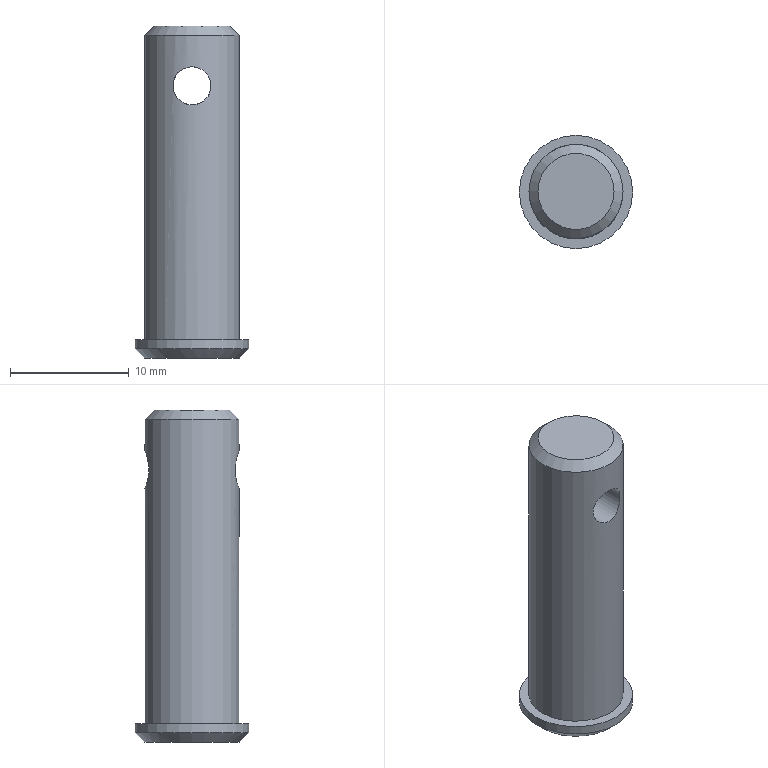Part | NX | features clevis pin, 312 2 | 1 solid | 8 faces | box 9.525 x 9.525 x 27.924 mm | volume 1333 mm3 | plane 3 | cylinder 3 | cone 2 | commonest cylinder face diameters 3.2 x1 7.925 x1 9.525 x1
STEP:
#1=CARTESIAN_POINT('',(4.763,0.,1.524));
#2=VERTEX_POINT('',#1);
#3=CARTESIAN_POINT('',(0.,0.,1.524));
#4=DIRECTION('',(0.,0.,1.));
#5=DIRECTION('',(1.,0.,0.));
#6=AXIS2_PLACEMENT_3D('',#3,#4,#5);
#7=CIRCLE('',#6,4.763);
#8=EDGE_CURVE('',#2,#2,#7,.T.);
#9=ORIENTED_EDGE('',*,*,#8,.T.);
#10=EDGE_LOOP('',(#9));
#11=FACE_BOUND('',#10,.T.);
#12=CARTESIAN_POINT('',(3.962,0.,1.524));
#13=VERTEX_POINT('',#12);
#14=CARTESIAN_POINT('',(0.,0.,1.524));
#15=DIRECTION('',(0.,0.,1.));
#16=DIRECTION('',(1.,0.,0.));
#17=AXIS2_PLACEMENT_3D('',#14,#15,#16);
#18=CIRCLE('',#17,3.962);
#19=EDGE_CURVE('',#13,#13,#18,.T.);
#20=ORIENTED_EDGE('',*,*,#19,.F.);
#21=EDGE_LOOP('',(#20));
#22=FACE_BOUND('',#21,.T.);
#23=CARTESIAN_POINT('',(0.,0.,1.524));
#24=DIRECTION('',(0.,0.,1.));
#25=DIRECTION('',(1.,0.,0.));
#26=AXIS2_PLACEMENT_3D('',#23,#24,#25);
#27=PLANE('',#26);
#28=ADVANCED_FACE('',(#11,#22),#27,.T.);
#29=CARTESIAN_POINT('',(4.763,0.,0.762));
#30=VERTEX_POINT('',#29);
#31=CARTESIAN_POINT('',(0.,0.,0.762));
#32=DIRECTION('',(0.,0.,1.));
#33=DIRECTION('',(1.,0.,0.));
#34=AXIS2_PLACEMENT_3D('',#31,#32,#33);
#35=CIRCLE('',#34,4.763);
#36=EDGE_CURVE('',#30,#30,#35,.T.);
#37=ORIENTED_EDGE('',*,*,#36,.T.);
#38=EDGE_LOOP('',(#37));
#39=FACE_BOUND('',#38,.T.);
#40=ORIENTED_EDGE('',*,*,#8,.F.);
#41=EDGE_LOOP('',(#40));
#42=FACE_BOUND('',#41,.T.);
#43=CARTESIAN_POINT('',(0.,0.,1.524));
#44=DIRECTION('',(0.,0.,-1.));
#45=DIRECTION('',(-1.,0.,0.));
#46=AXIS2_PLACEMENT_3D('',#43,#44,#45);
#47=CYLINDRICAL_SURFACE('',#46,4.763);
#48=ADVANCED_FACE('',(#39,#42),#47,.T.);
#49=CARTESIAN_POINT('',(4.,0.,0.));
#50=VERTEX_POINT('',#49);
#51=CARTESIAN_POINT('',(0.,0.,0.));
#52=DIRECTION('',(0.,0.,1.));
#53=DIRECTION('',(1.,0.,0.));
#54=AXIS2_PLACEMENT_3D('',#51,#52,#53);
#55=CIRCLE('',#54,4.);
#56=EDGE_CURVE('',#50,#50,#55,.F.);
#57=ORIENTED_EDGE('',*,*,#56,.T.);
#58=EDGE_LOOP('',(#57));
#59=FACE_BOUND('',#58,.T.);
#60=CARTESIAN_POINT('',(0.,0.,0.));
#61=DIRECTION('',(0.,0.,1.));
#62=DIRECTION('',(1.,0.,0.));
#63=AXIS2_PLACEMENT_3D('',#60,#61,#62);
#64=PLANE('',#63);
#65=ADVANCED_FACE('',(#59),#64,.F.);
#66=CARTESIAN_POINT('',(-0.4055,-3.942,24.44));
#67=VERTEX_POINT('',#66);
#68=CARTESIAN_POINT('',(-1.526,-3.676,23.796));
#69=CARTESIAN_POINT('',(-0.4535,-4.013,24.607));
#70=CARTESIAN_POINT('',(0.9067,-3.92,24.415));
#71=CARTESIAN_POINT('',(1.713,-3.572,23.348));
#72=CARTESIAN_POINT('',(1.524,-3.676,21.987));
#73=CARTESIAN_POINT('',(0.4564,-4.013,21.179));
#74=CARTESIAN_POINT('',(-0.906,-3.921,21.367));
#75=CARTESIAN_POINT('',(-1.713,-3.572,22.437));
#76=CARTESIAN_POINT('',(-1.526,-3.676,23.796));
#77=CARTESIAN_POINT('',(-0.4535,-4.013,24.607));
#78=CARTESIAN_POINT('',(0.9067,-3.92,24.415));
#79=B_SPLINE_CURVE_WITH_KNOTS('',3,(#68,#69,#70,#71,#72,#73,#74,#75,#76,#77,#78),.UNSPECIFIED.,.T.,.F.,(1,1,1,1,1,1,1,1,1,1,1,1,1,1,1),(-0.003793,-0.002529,-0.001264,0.,0.001264,0.002529,0.003793,0.005057,0.006321,0.007586,0.00885,0.01011,0.01138,0.01264,0.01391),.UNSPECIFIED.);
#80=EDGE_CURVE('',#67,#67,#79,.T.);
#81=ORIENTED_EDGE('',*,*,#80,.T.);
#82=EDGE_LOOP('',(#81));
#83=FACE_BOUND('',#82,.T.);
#84=CARTESIAN_POINT('',(0.4055,3.942,24.44));
#85=VERTEX_POINT('',#84);
#86=CARTESIAN_POINT('',(1.526,3.676,23.796));
#87=CARTESIAN_POINT('',(0.4535,4.013,24.607));
#88=CARTESIAN_POINT('',(-0.9067,3.92,24.415));
#89=CARTESIAN_POINT('',(-1.713,3.572,23.348));
#90=CARTESIAN_POINT('',(-1.524,3.676,21.987));
#91=CARTESIAN_POINT('',(-0.4564,4.013,21.179));
#92=CARTESIAN_POINT('',(0.906,3.921,21.367));
#93=CARTESIAN_POINT('',(1.713,3.572,22.437));
#94=CARTESIAN_POINT('',(1.526,3.676,23.796));
#95=CARTESIAN_POINT('',(0.4535,4.013,24.607));
#96=CARTESIAN_POINT('',(-0.9067,3.92,24.415));
#97=B_SPLINE_CURVE_WITH_KNOTS('',3,(#86,#87,#88,#89,#90,#91,#92,#93,#94,#95,#96),.UNSPECIFIED.,.T.,.F.,(1,1,1,1,1,1,1,1,1,1,1,1,1,1,1),(-0.003793,-0.002529,-0.001264,0.,0.001264,0.002529,0.003793,0.005057,0.006321,0.007586,0.00885,0.01011,0.01138,0.01264,0.01391),.UNSPECIFIED.);
#98=EDGE_CURVE('',#85,#85,#97,.T.);
#99=ORIENTED_EDGE('',*,*,#98,.T.);
#100=EDGE_LOOP('',(#99));
#101=FACE_BOUND('',#100,.T.);
#102=CARTESIAN_POINT('',(3.962,0.,27.162));
#103=VERTEX_POINT('',#102);
#104=CARTESIAN_POINT('',(0.,0.,27.162));
#105=DIRECTION('',(0.,0.,1.));
#106=DIRECTION('',(1.,0.,0.));
#107=AXIS2_PLACEMENT_3D('',#104,#105,#106);
#108=CIRCLE('',#107,3.962);
#109=EDGE_CURVE('',#103,#103,#108,.F.);
#110=ORIENTED_EDGE('',*,*,#109,.T.);
#111=EDGE_LOOP('',(#110));
#112=FACE_BOUND('',#111,.T.);
#113=ORIENTED_EDGE('',*,*,#19,.T.);
#114=EDGE_LOOP('',(#113));
#115=FACE_BOUND('',#114,.T.);
#116=CARTESIAN_POINT('',(0.,0.,26.924));
#117=DIRECTION('',(0.,0.,-1.));
#118=DIRECTION('',(-1.,0.,0.));
#119=AXIS2_PLACEMENT_3D('',#116,#117,#118);
#120=CYLINDRICAL_SURFACE('',#119,3.962);
#121=ADVANCED_FACE('',(#83,#101,#112,#115),#120,.T.);
#122=CARTESIAN_POINT('',(3.2,0.,27.924));
#123=VERTEX_POINT('',#122);
#124=CARTESIAN_POINT('',(0.,0.,27.924));
#125=DIRECTION('',(0.,0.,1.));
#126=DIRECTION('',(1.,0.,0.));
#127=AXIS2_PLACEMENT_3D('',#124,#125,#126);
#128=CIRCLE('',#127,3.2);
#129=EDGE_CURVE('',#123,#123,#128,.T.);
#130=ORIENTED_EDGE('',*,*,#129,.T.);
#131=EDGE_LOOP('',(#130));
#132=FACE_BOUND('',#131,.T.);
#133=CARTESIAN_POINT('',(0.,0.,27.924));
#134=DIRECTION('',(0.,0.,1.));
#135=DIRECTION('',(1.,0.,0.));
#136=AXIS2_PLACEMENT_3D('',#133,#134,#135);
#137=PLANE('',#136);
#138=ADVANCED_FACE('',(#132),#137,.T.);
#139=ORIENTED_EDGE('',*,*,#56,.F.);
#140=EDGE_LOOP('',(#139));
#141=FACE_BOUND('',#140,.T.);
#142=ORIENTED_EDGE('',*,*,#36,.F.);
#143=EDGE_LOOP('',(#142));
#144=FACE_BOUND('',#143,.T.);
#145=CARTESIAN_POINT('',(0.,0.,0.762));
#146=DIRECTION('',(0.,0.,1.));
#147=DIRECTION('',(1.,0.,0.));
#148=AXIS2_PLACEMENT_3D('',#145,#146,#147);
#149=CONICAL_SURFACE('',#148,4.763,0.7854);
#150=ADVANCED_FACE('',(#141,#144),#149,.T.);
#151=ORIENTED_EDGE('',*,*,#109,.F.);
#152=EDGE_LOOP('',(#151));
#153=FACE_BOUND('',#152,.T.);
#154=ORIENTED_EDGE('',*,*,#129,.F.);
#155=EDGE_LOOP('',(#154));
#156=FACE_BOUND('',#155,.T.);
#157=CARTESIAN_POINT('',(0.,0.,27.924));
#158=DIRECTION('',(0.,0.,-1.));
#159=DIRECTION('',(-1.,0.,0.));
#160=AXIS2_PLACEMENT_3D('',#157,#158,#159);
#161=CONICAL_SURFACE('',#160,3.2,0.7854);
#162=ADVANCED_FACE('',(#153,#156),#161,.T.);
#163=ORIENTED_EDGE('',*,*,#98,.F.);
#164=EDGE_LOOP('',(#163));
#165=FACE_BOUND('',#164,.T.);
#166=ORIENTED_EDGE('',*,*,#80,.F.);
#167=EDGE_LOOP('',(#166));
#168=FACE_BOUND('',#167,.T.);
#169=CARTESIAN_POINT('',(0.,-4.763,22.892));
#170=DIRECTION('',(0.,1.,0.));
#171=DIRECTION('',(0.,0.,1.));
#172=AXIS2_PLACEMENT_3D('',#169,#170,#171);
#173=CYLINDRICAL_SURFACE('',#172,1.6);
#174=ADVANCED_FACE('',(#165,#168),#173,.F.);
#175=CLOSED_SHELL('',(#28,#48,#65,#121,#138,#150,#162,#174));
#176=MANIFOLD_SOLID_BREP('',#175);
#177=(LENGTH_UNIT()NAMED_UNIT(*)SI_UNIT(.MILLI.,.METRE.));
#178=UNCERTAINTY_MEASURE_WITH_UNIT(LENGTH_MEASURE(0.0508),#177,'','');
#179=(NAMED_UNIT(*)PLANE_ANGLE_UNIT()SI_UNIT($,.RADIAN.));
#180=(NAMED_UNIT(*)SI_UNIT($,.STERADIAN.)SOLID_ANGLE_UNIT());
#181=(GEOMETRIC_REPRESENTATION_CONTEXT(3)GLOBAL_UNCERTAINTY_ASSIGNED_CONTEXT((#178))GLOBAL_UNIT_ASSIGNED_CONTEXT((#177,#179,#180))REPRESENTATION_CONTEXT('',''));
#182=ADVANCED_BREP_SHAPE_REPRESENTATION('',(#176),#181);